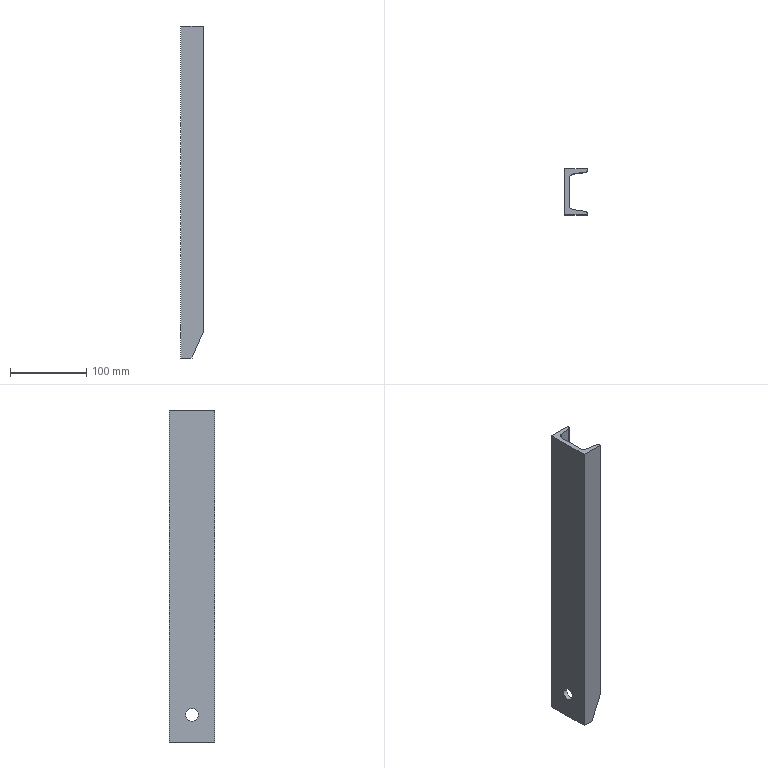Part | SolidWorks | features ICE 2, Extrusion 1 | 1 solid | 18 faces | box 30 x 60 x 435 mm | volume 273006 mm3 | plane 12 | cylinder 6 | commonest cylinder face diameters 6 x2 12 x2 17 x2
STEP:
#1=CARTESIAN_POINT('',(-24.,-21.5,35.5));
#2=VERTEX_POINT('',#1);
#3=CARTESIAN_POINT('',(-24.,-38.5,35.5));
#4=VERTEX_POINT('',#3);
#5=CARTESIAN_POINT('',(-24.,-30.,35.5));
#6=DIRECTION('',(-1.,0.,0.));
#7=DIRECTION('',(0.,0.,1.));
#8=AXIS2_PLACEMENT_3D('',#5,#6,#7);
#9=CIRCLE('',#8,8.5);
#10=EDGE_CURVE('',#2,#4,#9,.T.);
#11=ORIENTED_EDGE('',*,*,#10,.F.);
#12=CARTESIAN_POINT('',(-30.,-21.5,35.5));
#13=VERTEX_POINT('',#12);
#14=CARTESIAN_POINT('',(405.,-21.5,35.5));
#15=DIRECTION('',(-1.,0.,0.));
#16=VECTOR('',#15,1000.);
#17=LINE('',#14,#16);
#18=EDGE_CURVE('',#2,#13,#17,.T.);
#19=ORIENTED_EDGE('',*,*,#18,.T.);
#20=CARTESIAN_POINT('',(-30.,-38.5,35.5));
#21=VERTEX_POINT('',#20);
#22=CARTESIAN_POINT('',(-30.,-30.,35.5));
#23=DIRECTION('',(-1.,0.,0.));
#24=DIRECTION('',(0.,-1.,0.));
#25=AXIS2_PLACEMENT_3D('',#22,#23,#24);
#26=CIRCLE('',#25,8.5);
#27=EDGE_CURVE('',#13,#21,#26,.T.);
#28=ORIENTED_EDGE('',*,*,#27,.T.);
#29=CARTESIAN_POINT('',(405.,-38.5,35.5));
#30=DIRECTION('',(-1.,0.,0.));
#31=VECTOR('',#30,1000.);
#32=LINE('',#29,#31);
#33=EDGE_CURVE('',#4,#21,#32,.T.);
#34=ORIENTED_EDGE('',*,*,#33,.F.);
#35=EDGE_LOOP('',(#11,#19,#28,#34));
#36=FACE_OUTER_BOUND('',#35,.T.);
#37=CARTESIAN_POINT('',(405.,-30.,35.5));
#38=DIRECTION('',(-1.,0.,0.));
#39=DIRECTION('',(0.,-1.,0.));
#40=AXIS2_PLACEMENT_3D('',#37,#38,#39);
#41=CYLINDRICAL_SURFACE('',#40,8.5);
#42=ADVANCED_FACE('',(#36),#41,.F.);
#43=CARTESIAN_POINT('',(0.,-1.284,435.));
#44=VERTEX_POINT('',#43);
#45=CARTESIAN_POINT('',(0.,-1.284,35.));
#46=VERTEX_POINT('',#45);
#47=CARTESIAN_POINT('',(0.,-1.284,435.));
#48=DIRECTION('',(0.,0.,-1.));
#49=VECTOR('',#48,1000.);
#50=LINE('',#47,#49);
#51=EDGE_CURVE('',#44,#46,#50,.T.);
#52=ORIENTED_EDGE('',*,*,#51,.T.);
#53=CARTESIAN_POINT('',(0.,0.,35.));
#54=VERTEX_POINT('',#53);
#55=CARTESIAN_POINT('',(0.,-435.,35.));
#56=DIRECTION('',(0.,1.,0.));
#57=VECTOR('',#56,1000.);
#58=LINE('',#55,#57);
#59=EDGE_CURVE('',#46,#54,#58,.T.);
#60=ORIENTED_EDGE('',*,*,#59,.T.);
#61=CARTESIAN_POINT('',(0.,0.,435.));
#62=VERTEX_POINT('',#61);
#63=CARTESIAN_POINT('',(0.,0.,435.));
#64=DIRECTION('',(0.,0.,-1.));
#65=VECTOR('',#64,1000.);
#66=LINE('',#63,#65);
#67=EDGE_CURVE('',#62,#54,#66,.T.);
#68=ORIENTED_EDGE('',*,*,#67,.F.);
#69=CARTESIAN_POINT('',(0.,-1.284,435.));
#70=DIRECTION('',(0.,1.,0.));
#71=VECTOR('',#70,1000.);
#72=LINE('',#69,#71);
#73=EDGE_CURVE('',#44,#62,#72,.T.);
#74=ORIENTED_EDGE('',*,*,#73,.F.);
#75=EDGE_LOOP('',(#52,#60,#68,#74));
#76=FACE_OUTER_BOUND('',#75,.T.);
#77=CARTESIAN_POINT('',(0.,-1.284,435.));
#78=DIRECTION('',(-1.,0.,0.));
#79=DIRECTION('',(0.,0.,1.));
#80=AXIS2_PLACEMENT_3D('',#77,#78,#79);
#81=PLANE('',#80);
#82=ADVANCED_FACE('',(#76),#81,.F.);
#83=ORIENTED_EDGE('',*,*,#67,.T.);
#84=CARTESIAN_POINT('',(-15.,0.,0.));
#85=VERTEX_POINT('',#84);
#86=CARTESIAN_POINT('',(0.,0.,35.));
#87=DIRECTION('',(0.3939,0.,0.9191));
#88=VECTOR('',#87,1000.);
#89=LINE('',#86,#88);
#90=EDGE_CURVE('',#85,#54,#89,.T.);
#91=ORIENTED_EDGE('',*,*,#90,.F.);
#92=CARTESIAN_POINT('',(-30.,0.,0.));
#93=VERTEX_POINT('',#92);
#94=CARTESIAN_POINT('',(0.,0.,0.));
#95=DIRECTION('',(-1.,0.,0.));
#96=VECTOR('',#95,1000.);
#97=LINE('',#94,#96);
#98=EDGE_CURVE('',#85,#93,#97,.T.);
#99=ORIENTED_EDGE('',*,*,#98,.T.);
#100=CARTESIAN_POINT('',(-30.,0.,435.));
#101=VERTEX_POINT('',#100);
#102=CARTESIAN_POINT('',(-30.,0.,435.));
#103=DIRECTION('',(0.,0.,-1.));
#104=VECTOR('',#103,1000.);
#105=LINE('',#102,#104);
#106=EDGE_CURVE('',#101,#93,#105,.T.);
#107=ORIENTED_EDGE('',*,*,#106,.F.);
#108=CARTESIAN_POINT('',(0.,0.,435.));
#109=DIRECTION('',(-1.,0.,0.));
#110=VECTOR('',#109,1000.);
#111=LINE('',#108,#110);
#112=EDGE_CURVE('',#62,#101,#111,.T.);
#113=ORIENTED_EDGE('',*,*,#112,.F.);
#114=EDGE_LOOP('',(#83,#91,#99,#107,#113));
#115=FACE_OUTER_BOUND('',#114,.T.);
#116=CARTESIAN_POINT('',(0.,0.,435.));
#117=DIRECTION('',(0.,-1.,0.));
#118=DIRECTION('',(1.,0.,0.));
#119=AXIS2_PLACEMENT_3D('',#116,#117,#118);
#120=PLANE('',#119);
#121=ADVANCED_FACE('',(#115),#120,.F.);
#122=CARTESIAN_POINT('',(-30.,-30.,35.5));
#123=DIRECTION('',(-1.,0.,0.));
#124=DIRECTION('',(0.,-1.,0.));
#125=AXIS2_PLACEMENT_3D('',#122,#123,#124);
#126=CIRCLE('',#125,8.5);
#127=EDGE_CURVE('',#21,#13,#126,.T.);
#128=ORIENTED_EDGE('',*,*,#127,.F.);
#129=ORIENTED_EDGE('',*,*,#27,.F.);
#130=EDGE_LOOP('',(#128,#129));
#131=FACE_BOUND('',#130,.T.);
#132=CARTESIAN_POINT('',(-30.,-60.,0.));
#133=VERTEX_POINT('',#132);
#134=CARTESIAN_POINT('',(-30.,0.,0.));
#135=DIRECTION('',(0.,-1.,0.));
#136=VECTOR('',#135,1000.);
#137=LINE('',#134,#136);
#138=EDGE_CURVE('',#93,#133,#137,.T.);
#139=ORIENTED_EDGE('',*,*,#138,.T.);
#140=CARTESIAN_POINT('',(-30.,-60.,435.));
#141=VERTEX_POINT('',#140);
#142=CARTESIAN_POINT('',(-30.,-60.,435.));
#143=DIRECTION('',(0.,0.,-1.));
#144=VECTOR('',#143,1000.);
#145=LINE('',#142,#144);
#146=EDGE_CURVE('',#141,#133,#145,.T.);
#147=ORIENTED_EDGE('',*,*,#146,.F.);
#148=CARTESIAN_POINT('',(-30.,0.,435.));
#149=DIRECTION('',(0.,-1.,0.));
#150=VECTOR('',#149,1000.);
#151=LINE('',#148,#150);
#152=EDGE_CURVE('',#101,#141,#151,.T.);
#153=ORIENTED_EDGE('',*,*,#152,.F.);
#154=ORIENTED_EDGE('',*,*,#106,.T.);
#155=EDGE_LOOP('',(#139,#147,#153,#154));
#156=FACE_OUTER_BOUND('',#155,.T.);
#157=CARTESIAN_POINT('',(-30.,0.,435.));
#158=DIRECTION('',(1.,0.,0.));
#159=DIRECTION('',(0.,1.,0.));
#160=AXIS2_PLACEMENT_3D('',#157,#158,#159);
#161=PLANE('',#160);
#162=ADVANCED_FACE('',(#131,#156),#161,.F.);
#163=CARTESIAN_POINT('',(-15.,-60.,0.));
#164=VERTEX_POINT('',#163);
#165=CARTESIAN_POINT('',(-30.,-60.,0.));
#166=DIRECTION('',(1.,0.,0.));
#167=VECTOR('',#166,1000.);
#168=LINE('',#165,#167);
#169=EDGE_CURVE('',#133,#164,#168,.T.);
#170=ORIENTED_EDGE('',*,*,#169,.T.);
#171=CARTESIAN_POINT('',(0.,-60.,35.));
#172=VERTEX_POINT('',#171);
#173=CARTESIAN_POINT('',(140.172,-60.,362.069));
#174=DIRECTION('',(0.3939,0.,0.9191));
#175=VECTOR('',#174,1000.);
#176=LINE('',#173,#175);
#177=EDGE_CURVE('',#164,#172,#176,.T.);
#178=ORIENTED_EDGE('',*,*,#177,.T.);
#179=CARTESIAN_POINT('',(0.,-60.,435.));
#180=VERTEX_POINT('',#179);
#181=CARTESIAN_POINT('',(0.,-60.,435.));
#182=DIRECTION('',(0.,0.,-1.));
#183=VECTOR('',#182,1000.);
#184=LINE('',#181,#183);
#185=EDGE_CURVE('',#180,#172,#184,.T.);
#186=ORIENTED_EDGE('',*,*,#185,.F.);
#187=CARTESIAN_POINT('',(-30.,-60.,435.));
#188=DIRECTION('',(1.,0.,0.));
#189=VECTOR('',#188,1000.);
#190=LINE('',#187,#189);
#191=EDGE_CURVE('',#141,#180,#190,.T.);
#192=ORIENTED_EDGE('',*,*,#191,.F.);
#193=ORIENTED_EDGE('',*,*,#146,.T.);
#194=EDGE_LOOP('',(#170,#178,#186,#192,#193));
#195=FACE_OUTER_BOUND('',#194,.T.);
#196=CARTESIAN_POINT('',(-30.,-60.,435.));
#197=DIRECTION('',(0.,1.,0.));
#198=DIRECTION('',(-1.,0.,0.));
#199=AXIS2_PLACEMENT_3D('',#196,#197,#198);
#200=PLANE('',#199);
#201=ADVANCED_FACE('',(#195),#200,.F.);
#202=ORIENTED_EDGE('',*,*,#185,.T.);
#203=CARTESIAN_POINT('',(0.,-58.716,35.));
#204=VERTEX_POINT('',#203);
#205=CARTESIAN_POINT('',(0.,-435.,35.));
#206=DIRECTION('',(0.,1.,0.));
#207=VECTOR('',#206,1000.);
#208=LINE('',#205,#207);
#209=EDGE_CURVE('',#172,#204,#208,.T.);
#210=ORIENTED_EDGE('',*,*,#209,.T.);
#211=CARTESIAN_POINT('',(0.,-58.716,435.));
#212=VERTEX_POINT('',#211);
#213=CARTESIAN_POINT('',(0.,-58.716,435.));
#214=DIRECTION('',(0.,0.,-1.));
#215=VECTOR('',#214,1000.);
#216=LINE('',#213,#215);
#217=EDGE_CURVE('',#212,#204,#216,.T.);
#218=ORIENTED_EDGE('',*,*,#217,.F.);
#219=CARTESIAN_POINT('',(0.,-60.,435.));
#220=DIRECTION('',(0.,1.,0.));
#221=VECTOR('',#220,1000.);
#222=LINE('',#219,#221);
#223=EDGE_CURVE('',#180,#212,#222,.T.);
#224=ORIENTED_EDGE('',*,*,#223,.F.);
#225=EDGE_LOOP('',(#202,#210,#218,#224));
#226=FACE_OUTER_BOUND('',#225,.T.);
#227=CARTESIAN_POINT('',(0.,-60.,435.));
#228=DIRECTION('',(-1.,0.,0.));
#229=DIRECTION('',(0.,0.,1.));
#230=AXIS2_PLACEMENT_3D('',#227,#228,#229);
#231=PLANE('',#230);
#232=ADVANCED_FACE('',(#226),#231,.F.);
#233=ORIENTED_EDGE('',*,*,#217,.T.);
#234=CARTESIAN_POINT('',(-2.582,-55.745,28.974));
#235=VERTEX_POINT('',#234);
#236=CARTESIAN_POINT('',(0.,-58.716,35.));
#237=CARTESIAN_POINT('',(0.,-57.147,35.));
#238=CARTESIAN_POINT('',(-1.029,-55.963,32.599));
#239=CARTESIAN_POINT('',(-2.582,-55.745,28.974));
#240=(BOUNDED_CURVE()B_SPLINE_CURVE(3,(#236,#237,#238,#239),.UNSPECIFIED.,.F.,.T.)B_SPLINE_CURVE_WITH_KNOTS((4,4),(3.142,4.573),.UNSPECIFIED.)CURVE()GEOMETRIC_REPRESENTATION_ITEM()RATIONAL_B_SPLINE_CURVE((1.,0.8365,0.8365,1.))REPRESENTATION_ITEM(''));
#241=EDGE_CURVE('',#204,#235,#240,.T.);
#242=ORIENTED_EDGE('',*,*,#241,.T.);
#243=CARTESIAN_POINT('',(-2.582,-55.745,435.));
#244=VERTEX_POINT('',#243);
#245=CARTESIAN_POINT('',(-2.582,-55.745,435.));
#246=DIRECTION('',(0.,0.,-1.));
#247=VECTOR('',#246,1000.);
#248=LINE('',#245,#247);
#249=EDGE_CURVE('',#244,#235,#248,.T.);
#250=ORIENTED_EDGE('',*,*,#249,.F.);
#251=CARTESIAN_POINT('',(-3.,-58.716,435.));
#252=DIRECTION('',(0.,0.,1.));
#253=DIRECTION('',(1.,0.,0.));
#254=AXIS2_PLACEMENT_3D('',#251,#252,#253);
#255=CIRCLE('',#254,3.);
#256=EDGE_CURVE('',#212,#244,#255,.T.);
#257=ORIENTED_EDGE('',*,*,#256,.F.);
#258=EDGE_LOOP('',(#233,#242,#250,#257));
#259=FACE_OUTER_BOUND('',#258,.T.);
#260=CARTESIAN_POINT('',(-3.,-58.716,435.));
#261=DIRECTION('',(0.,0.,-1.));
#262=DIRECTION('',(-1.,0.,0.));
#263=AXIS2_PLACEMENT_3D('',#260,#261,#262);
#264=CYLINDRICAL_SURFACE('',#263,3.);
#265=ADVANCED_FACE('',(#259),#264,.T.);
#266=ORIENTED_EDGE('',*,*,#249,.T.);
#267=CARTESIAN_POINT('',(-15.,-54.,0.));
#268=VERTEX_POINT('',#267);
#269=CARTESIAN_POINT('',(143.978,-76.343,370.948));
#270=DIRECTION('',(-0.3933,0.05528,-0.9177));
#271=VECTOR('',#270,1000.);
#272=LINE('',#269,#271);
#273=EDGE_CURVE('',#235,#268,#272,.T.);
#274=ORIENTED_EDGE('',*,*,#273,.T.);
#275=CARTESIAN_POINT('',(-18.835,-53.461,0.));
#276=VERTEX_POINT('',#275);
#277=CARTESIAN_POINT('',(-2.582,-55.745,0.));
#278=DIRECTION('',(-0.9903,0.1392,0.));
#279=VECTOR('',#278,1000.);
#280=LINE('',#277,#279);
#281=EDGE_CURVE('',#268,#276,#280,.T.);
#282=ORIENTED_EDGE('',*,*,#281,.T.);
#283=CARTESIAN_POINT('',(-18.835,-53.461,435.));
#284=VERTEX_POINT('',#283);
#285=CARTESIAN_POINT('',(-18.835,-53.461,435.));
#286=DIRECTION('',(0.,0.,-1.));
#287=VECTOR('',#286,1000.);
#288=LINE('',#285,#287);
#289=EDGE_CURVE('',#284,#276,#288,.T.);
#290=ORIENTED_EDGE('',*,*,#289,.F.);
#291=CARTESIAN_POINT('',(-2.582,-55.745,435.));
#292=DIRECTION('',(-0.9903,0.1392,0.));
#293=VECTOR('',#292,1000.);
#294=LINE('',#291,#293);
#295=EDGE_CURVE('',#244,#284,#294,.T.);
#296=ORIENTED_EDGE('',*,*,#295,.F.);
#297=EDGE_LOOP('',(#266,#274,#282,#290,#296));
#298=FACE_OUTER_BOUND('',#297,.T.);
#299=CARTESIAN_POINT('',(-2.582,-55.745,435.));
#300=DIRECTION('',(-0.1392,-0.9903,0.));
#301=DIRECTION('',(0.9903,-0.1392,0.));
#302=AXIS2_PLACEMENT_3D('',#299,#300,#301);
#303=PLANE('',#302);
#304=ADVANCED_FACE('',(#298),#303,.F.);
#305=CARTESIAN_POINT('',(-24.,-47.519,0.));
#306=VERTEX_POINT('',#305);
#307=CARTESIAN_POINT('',(-18.,-47.519,0.));
#308=DIRECTION('',(0.,0.,-1.));
#309=DIRECTION('',(-1.,0.,0.));
#310=AXIS2_PLACEMENT_3D('',#307,#308,#309);
#311=CIRCLE('',#310,6.);
#312=EDGE_CURVE('',#276,#306,#311,.T.);
#313=ORIENTED_EDGE('',*,*,#312,.T.);
#314=CARTESIAN_POINT('',(-24.,-47.519,435.));
#315=VERTEX_POINT('',#314);
#316=CARTESIAN_POINT('',(-24.,-47.519,435.));
#317=DIRECTION('',(0.,0.,-1.));
#318=VECTOR('',#317,1000.);
#319=LINE('',#316,#318);
#320=EDGE_CURVE('',#315,#306,#319,.T.);
#321=ORIENTED_EDGE('',*,*,#320,.F.);
#322=CARTESIAN_POINT('',(-18.,-47.519,435.));
#323=DIRECTION('',(0.,0.,-1.));
#324=DIRECTION('',(-1.,0.,0.));
#325=AXIS2_PLACEMENT_3D('',#322,#323,#324);
#326=CIRCLE('',#325,6.);
#327=EDGE_CURVE('',#284,#315,#326,.T.);
#328=ORIENTED_EDGE('',*,*,#327,.F.);
#329=ORIENTED_EDGE('',*,*,#289,.T.);
#330=EDGE_LOOP('',(#313,#321,#328,#329));
#331=FACE_OUTER_BOUND('',#330,.T.);
#332=CARTESIAN_POINT('',(-18.,-47.519,435.));
#333=DIRECTION('',(0.,0.,-1.));
#334=DIRECTION('',(-1.,0.,0.));
#335=AXIS2_PLACEMENT_3D('',#332,#333,#334);
#336=CYLINDRICAL_SURFACE('',#335,6.);
#337=ADVANCED_FACE('',(#331),#336,.F.);
#338=CARTESIAN_POINT('',(-24.,-30.,35.5));
#339=DIRECTION('',(-1.,0.,0.));
#340=DIRECTION('',(0.,0.,1.));
#341=AXIS2_PLACEMENT_3D('',#338,#339,#340);
#342=CIRCLE('',#341,8.5);
#343=EDGE_CURVE('',#4,#2,#342,.T.);
#344=ORIENTED_EDGE('',*,*,#343,.T.);
#345=ORIENTED_EDGE('',*,*,#10,.T.);
#346=EDGE_LOOP('',(#344,#345));
#347=FACE_BOUND('',#346,.T.);
#348=CARTESIAN_POINT('',(-24.,-12.481,0.));
#349=VERTEX_POINT('',#348);
#350=CARTESIAN_POINT('',(-24.,-47.519,0.));
#351=DIRECTION('',(0.,1.,0.));
#352=VECTOR('',#351,1000.);
#353=LINE('',#350,#352);
#354=EDGE_CURVE('',#306,#349,#353,.T.);
#355=ORIENTED_EDGE('',*,*,#354,.T.);
#356=CARTESIAN_POINT('',(-24.,-12.481,435.));
#357=VERTEX_POINT('',#356);
#358=CARTESIAN_POINT('',(-24.,-12.481,435.));
#359=DIRECTION('',(0.,0.,-1.));
#360=VECTOR('',#359,1000.);
#361=LINE('',#358,#360);
#362=EDGE_CURVE('',#357,#349,#361,.T.);
#363=ORIENTED_EDGE('',*,*,#362,.F.);
#364=CARTESIAN_POINT('',(-24.,-47.519,435.));
#365=DIRECTION('',(0.,1.,0.));
#366=VECTOR('',#365,1000.);
#367=LINE('',#364,#366);
#368=EDGE_CURVE('',#315,#357,#367,.T.);
#369=ORIENTED_EDGE('',*,*,#368,.F.);
#370=ORIENTED_EDGE('',*,*,#320,.T.);
#371=EDGE_LOOP('',(#355,#363,#369,#370));
#372=FACE_OUTER_BOUND('',#371,.T.);
#373=CARTESIAN_POINT('',(-24.,-47.519,435.));
#374=DIRECTION('',(-1.,0.,0.));
#375=DIRECTION('',(0.,0.,1.));
#376=AXIS2_PLACEMENT_3D('',#373,#374,#375);
#377=PLANE('',#376);
#378=ADVANCED_FACE('',(#347,#372),#377,.F.);
#379=CARTESIAN_POINT('',(-18.835,-6.539,0.));
#380=VERTEX_POINT('',#379);
#381=CARTESIAN_POINT('',(-18.,-12.481,0.));
#382=DIRECTION('',(0.,0.,-1.));
#383=DIRECTION('',(-1.,0.,0.));
#384=AXIS2_PLACEMENT_3D('',#381,#382,#383);
#385=CIRCLE('',#384,6.);
#386=EDGE_CURVE('',#349,#380,#385,.T.);
#387=ORIENTED_EDGE('',*,*,#386,.T.);
#388=CARTESIAN_POINT('',(-18.835,-6.539,435.));
#389=VERTEX_POINT('',#388);
#390=CARTESIAN_POINT('',(-18.835,-6.539,435.));
#391=DIRECTION('',(0.,0.,-1.));
#392=VECTOR('',#391,1000.);
#393=LINE('',#390,#392);
#394=EDGE_CURVE('',#389,#380,#393,.T.);
#395=ORIENTED_EDGE('',*,*,#394,.F.);
#396=CARTESIAN_POINT('',(-18.,-12.481,435.));
#397=DIRECTION('',(0.,0.,-1.));
#398=DIRECTION('',(-1.,0.,0.));
#399=AXIS2_PLACEMENT_3D('',#396,#397,#398);
#400=CIRCLE('',#399,6.);
#401=EDGE_CURVE('',#357,#389,#400,.T.);
#402=ORIENTED_EDGE('',*,*,#401,.F.);
#403=ORIENTED_EDGE('',*,*,#362,.T.);
#404=EDGE_LOOP('',(#387,#395,#402,#403));
#405=FACE_OUTER_BOUND('',#404,.T.);
#406=CARTESIAN_POINT('',(-18.,-12.481,435.));
#407=DIRECTION('',(0.,0.,-1.));
#408=DIRECTION('',(-1.,0.,0.));
#409=AXIS2_PLACEMENT_3D('',#406,#407,#408);
#410=CYLINDRICAL_SURFACE('',#409,6.);
#411=ADVANCED_FACE('',(#405),#410,.F.);
#412=CARTESIAN_POINT('',(-15.,-6.,0.));
#413=VERTEX_POINT('',#412);
#414=CARTESIAN_POINT('',(-18.835,-6.539,0.));
#415=DIRECTION('',(0.9903,0.1392,0.));
#416=VECTOR('',#415,1000.);
#417=LINE('',#414,#416);
#418=EDGE_CURVE('',#380,#413,#417,.T.);
#419=ORIENTED_EDGE('',*,*,#418,.T.);
#420=CARTESIAN_POINT('',(-2.582,-4.255,28.974));
#421=VERTEX_POINT('',#420);
#422=CARTESIAN_POINT('',(141.414,15.983,364.965));
#423=DIRECTION('',(0.3933,0.05528,0.9177));
#424=VECTOR('',#423,1000.);
#425=LINE('',#422,#424);
#426=EDGE_CURVE('',#413,#421,#425,.T.);
#427=ORIENTED_EDGE('',*,*,#426,.T.);
#428=CARTESIAN_POINT('',(-2.582,-4.255,435.));
#429=VERTEX_POINT('',#428);
#430=CARTESIAN_POINT('',(-2.582,-4.255,435.));
#431=DIRECTION('',(0.,0.,-1.));
#432=VECTOR('',#431,1000.);
#433=LINE('',#430,#432);
#434=EDGE_CURVE('',#429,#421,#433,.T.);
#435=ORIENTED_EDGE('',*,*,#434,.F.);
#436=CARTESIAN_POINT('',(-18.835,-6.539,435.));
#437=DIRECTION('',(0.9903,0.1392,0.));
#438=VECTOR('',#437,1000.);
#439=LINE('',#436,#438);
#440=EDGE_CURVE('',#389,#429,#439,.T.);
#441=ORIENTED_EDGE('',*,*,#440,.F.);
#442=ORIENTED_EDGE('',*,*,#394,.T.);
#443=EDGE_LOOP('',(#419,#427,#435,#441,#442));
#444=FACE_OUTER_BOUND('',#443,.T.);
#445=CARTESIAN_POINT('',(-18.835,-6.539,435.));
#446=DIRECTION('',(-0.1392,0.9903,0.));
#447=DIRECTION('',(-0.9903,-0.1392,0.));
#448=AXIS2_PLACEMENT_3D('',#445,#446,#447);
#449=PLANE('',#448);
#450=ADVANCED_FACE('',(#444),#449,.F.);
#451=CARTESIAN_POINT('',(0.,-1.284,35.));
#452=CARTESIAN_POINT('',(0.,-2.853,35.));
#453=CARTESIAN_POINT('',(-1.029,-4.037,32.599));
#454=CARTESIAN_POINT('',(-2.582,-4.255,28.974));
#455=(BOUNDED_CURVE()B_SPLINE_CURVE(3,(#451,#452,#453,#454),.UNSPECIFIED.,.F.,.F.)B_SPLINE_CURVE_WITH_KNOTS((4,4),(3.142,4.573),.UNSPECIFIED.)CURVE()GEOMETRIC_REPRESENTATION_ITEM()RATIONAL_B_SPLINE_CURVE((1.,0.8365,0.8365,1.))REPRESENTATION_ITEM(''));
#456=EDGE_CURVE('',#46,#421,#455,.T.);
#457=ORIENTED_EDGE('',*,*,#456,.F.);
#458=ORIENTED_EDGE('',*,*,#51,.F.);
#459=CARTESIAN_POINT('',(-3.,-1.284,435.));
#460=DIRECTION('',(0.,0.,-1.));
#461=DIRECTION('',(-1.,0.,0.));
#462=AXIS2_PLACEMENT_3D('',#459,#460,#461);
#463=CIRCLE('',#462,3.);
#464=EDGE_CURVE('',#44,#429,#463,.T.);
#465=ORIENTED_EDGE('',*,*,#464,.T.);
#466=ORIENTED_EDGE('',*,*,#434,.T.);
#467=EDGE_LOOP('',(#457,#458,#465,#466));
#468=FACE_OUTER_BOUND('',#467,.T.);
#469=CARTESIAN_POINT('',(-3.,-1.284,435.));
#470=DIRECTION('',(0.,0.,-1.));
#471=DIRECTION('',(-1.,0.,0.));
#472=AXIS2_PLACEMENT_3D('',#469,#470,#471);
#473=CYLINDRICAL_SURFACE('',#472,3.);
#474=ADVANCED_FACE('',(#468),#473,.T.);
#475=ORIENTED_EDGE('',*,*,#73,.T.);
#476=ORIENTED_EDGE('',*,*,#112,.T.);
#477=ORIENTED_EDGE('',*,*,#152,.T.);
#478=ORIENTED_EDGE('',*,*,#191,.T.);
#479=ORIENTED_EDGE('',*,*,#223,.T.);
#480=ORIENTED_EDGE('',*,*,#256,.T.);
#481=ORIENTED_EDGE('',*,*,#295,.T.);
#482=ORIENTED_EDGE('',*,*,#327,.T.);
#483=ORIENTED_EDGE('',*,*,#368,.T.);
#484=ORIENTED_EDGE('',*,*,#401,.T.);
#485=ORIENTED_EDGE('',*,*,#440,.T.);
#486=ORIENTED_EDGE('',*,*,#464,.F.);
#487=EDGE_LOOP('',(#475,#476,#477,#478,#479,#480,#481,#482,#483,#484,#485,#486));
#488=FACE_OUTER_BOUND('',#487,.T.);
#489=CARTESIAN_POINT('',(-3.,-58.716,435.));
#490=DIRECTION('',(0.,0.,1.));
#491=DIRECTION('',(1.,0.,0.));
#492=AXIS2_PLACEMENT_3D('',#489,#490,#491);
#493=PLANE('',#492);
#494=ADVANCED_FACE('',(#488),#493,.T.);
#495=ORIENTED_EDGE('',*,*,#98,.F.);
#496=CARTESIAN_POINT('',(-15.,-58.716,0.));
#497=DIRECTION('',(0.,-1.,0.));
#498=VECTOR('',#497,1000.);
#499=LINE('',#496,#498);
#500=EDGE_CURVE('',#85,#413,#499,.T.);
#501=ORIENTED_EDGE('',*,*,#500,.T.);
#502=ORIENTED_EDGE('',*,*,#418,.F.);
#503=ORIENTED_EDGE('',*,*,#386,.F.);
#504=ORIENTED_EDGE('',*,*,#354,.F.);
#505=ORIENTED_EDGE('',*,*,#312,.F.);
#506=ORIENTED_EDGE('',*,*,#281,.F.);
#507=CARTESIAN_POINT('',(-15.,-58.716,0.));
#508=DIRECTION('',(0.,-1.,0.));
#509=VECTOR('',#508,1000.);
#510=LINE('',#507,#509);
#511=EDGE_CURVE('',#268,#164,#510,.T.);
#512=ORIENTED_EDGE('',*,*,#511,.T.);
#513=ORIENTED_EDGE('',*,*,#169,.F.);
#514=ORIENTED_EDGE('',*,*,#138,.F.);
#515=EDGE_LOOP('',(#495,#501,#502,#503,#504,#505,#506,#512,#513,#514));
#516=FACE_OUTER_BOUND('',#515,.T.);
#517=CARTESIAN_POINT('',(-3.,-58.716,0.));
#518=DIRECTION('',(0.,0.,1.));
#519=DIRECTION('',(1.,0.,0.));
#520=AXIS2_PLACEMENT_3D('',#517,#518,#519);
#521=PLANE('',#520);
#522=ADVANCED_FACE('',(#516),#521,.F.);
#523=ORIENTED_EDGE('',*,*,#18,.F.);
#524=ORIENTED_EDGE('',*,*,#343,.F.);
#525=ORIENTED_EDGE('',*,*,#33,.T.);
#526=ORIENTED_EDGE('',*,*,#127,.T.);
#527=EDGE_LOOP('',(#523,#524,#525,#526));
#528=FACE_OUTER_BOUND('',#527,.T.);
#529=CARTESIAN_POINT('',(405.,-30.,35.5));
#530=DIRECTION('',(-1.,0.,0.));
#531=DIRECTION('',(0.,-1.,0.));
#532=AXIS2_PLACEMENT_3D('',#529,#530,#531);
#533=CYLINDRICAL_SURFACE('',#532,8.5);
#534=ADVANCED_FACE('',(#528),#533,.F.);
#535=ORIENTED_EDGE('',*,*,#511,.F.);
#536=ORIENTED_EDGE('',*,*,#273,.F.);
#537=ORIENTED_EDGE('',*,*,#241,.F.);
#538=ORIENTED_EDGE('',*,*,#209,.F.);
#539=ORIENTED_EDGE('',*,*,#177,.F.);
#540=EDGE_LOOP('',(#535,#536,#537,#538,#539));
#541=FACE_OUTER_BOUND('',#540,.T.);
#542=CARTESIAN_POINT('',(0.,-435.,35.));
#543=DIRECTION('',(-0.9191,0.,0.3939));
#544=DIRECTION('',(0.3939,0.,0.9191));
#545=AXIS2_PLACEMENT_3D('',#542,#543,#544);
#546=PLANE('',#545);
#547=ADVANCED_FACE('',(#541),#546,.F.);
#548=ORIENTED_EDGE('',*,*,#500,.F.);
#549=ORIENTED_EDGE('',*,*,#90,.T.);
#550=ORIENTED_EDGE('',*,*,#59,.F.);
#551=ORIENTED_EDGE('',*,*,#456,.T.);
#552=ORIENTED_EDGE('',*,*,#426,.F.);
#553=EDGE_LOOP('',(#548,#549,#550,#551,#552));
#554=FACE_OUTER_BOUND('',#553,.T.);
#555=CARTESIAN_POINT('',(0.,-435.,35.));
#556=DIRECTION('',(-0.9191,0.,0.3939));
#557=DIRECTION('',(0.3939,0.,0.9191));
#558=AXIS2_PLACEMENT_3D('',#555,#556,#557);
#559=PLANE('',#558);
#560=ADVANCED_FACE('',(#554),#559,.F.);
#561=CLOSED_SHELL('',(#42,#82,#121,#162,#201,#232,#265,#304,#337,#378,#411,#450,#474,#494,#522,#534,#547,#560));
#562=MANIFOLD_SOLID_BREP('',#561);
#563=CARTESIAN_POINT('',(0.,0.,0.));
#564=DIRECTION('',(0.,0.,1.));
#565=DIRECTION('',(1.,0.,0.));
#566=AXIS2_PLACEMENT_3D('',#563,#564,#565);
#567=(LENGTH_UNIT()NAMED_UNIT(*)SI_UNIT(.MILLI.,.METRE.));
#568=UNCERTAINTY_MEASURE_WITH_UNIT(LENGTH_MEASURE(0.00001),#567,'','');
#569=(NAMED_UNIT(*)PLANE_ANGLE_UNIT()SI_UNIT($,.RADIAN.));
#570=(NAMED_UNIT(*)SI_UNIT($,.STERADIAN.)SOLID_ANGLE_UNIT());
#571=(GEOMETRIC_REPRESENTATION_CONTEXT(3)GLOBAL_UNCERTAINTY_ASSIGNED_CONTEXT((#568))GLOBAL_UNIT_ASSIGNED_CONTEXT((#567,#569,#570))REPRESENTATION_CONTEXT('',''));
#572=ADVANCED_BREP_SHAPE_REPRESENTATION('',(#562,#566),#571);